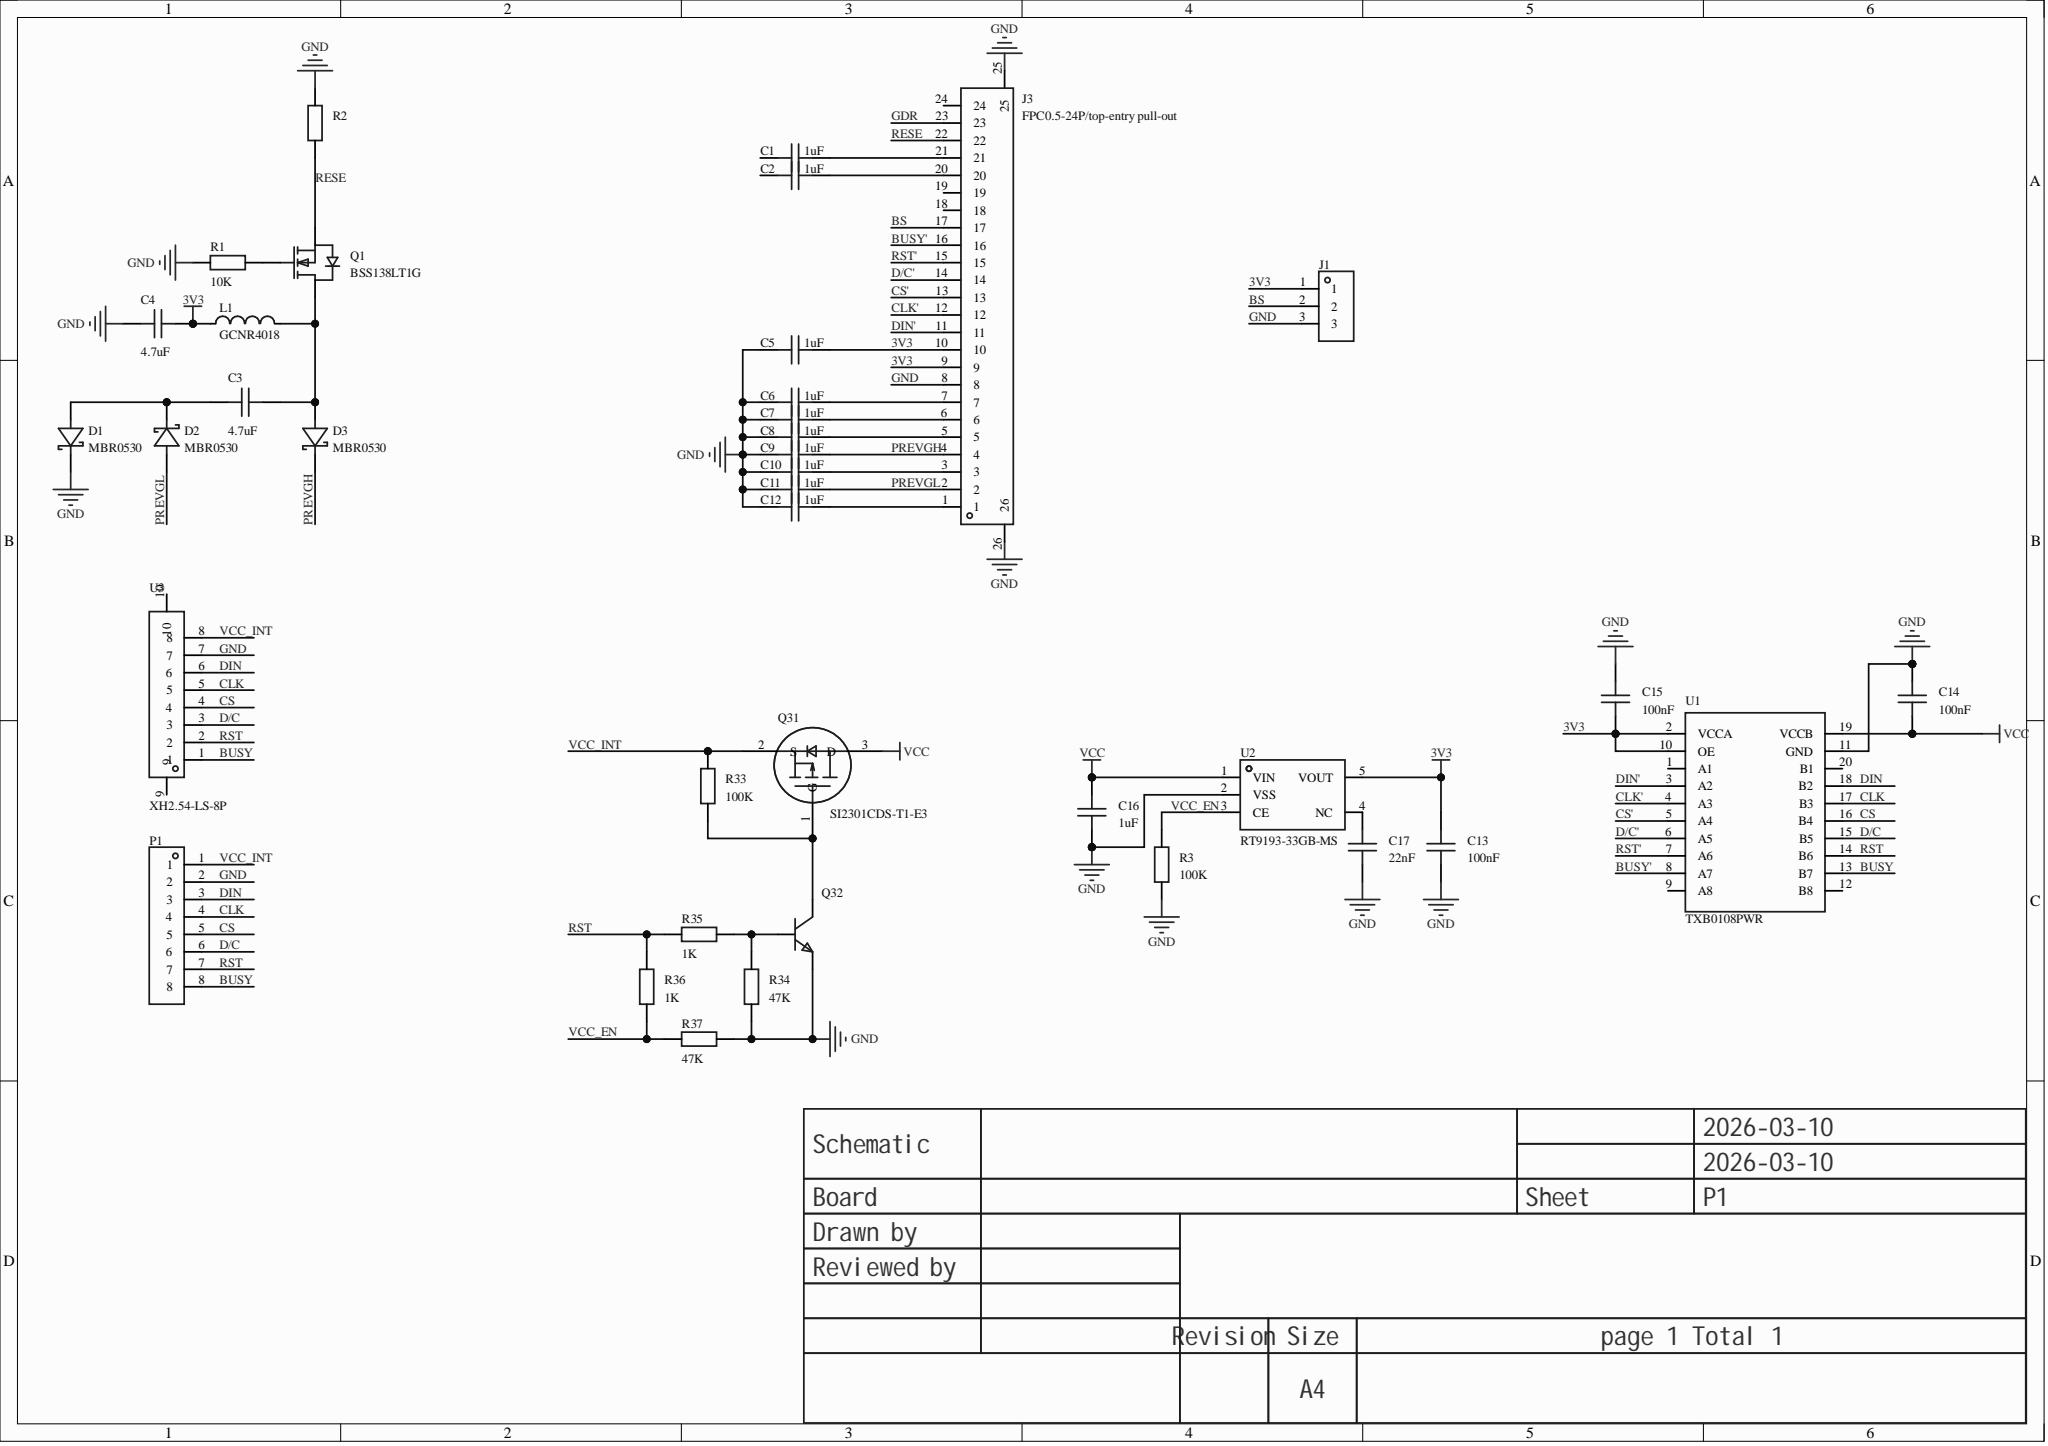Circuit board | Altium Designer | 38 parts | 34 nets
Bill of materials:
Comment,Description,Designator,Footprint,LibRef,Quantity
"1uF","","C1, C2, C5, C6, C7, C8, C9, C10, C11, C12, C16","C0603","CAP_0603","11"
"4.7uF","","C3, C4","C0603","CAP_0603","2"
"100nF","","C13, C14, C15","C0603","CAP_0603","3"
"22nF","","C17","C0603","CAP_0603","1"
"MBR0530","Diode configuration: single; forward voltage (Vf): 550mV@500mA; DC reverse voltage (Vr): 30V; rectified current: 500mA;","D1, D2, D3","SOD-123FL_L2.7-W1.8-LS3.7-RD","MBR0530","3"
"","","J1","HDR-TH_3P-P2.54-V-F","HDR-F_2.54_1x3P","1"
"FPC0.5-24P/top-entry pull-out","","J3","FPC-SMD_24P-P0.50_SHOU-HAN_CTSJ-H2.0","FPC0.5-24P/上接抽拉","1"
"GCNR4018","","L1","IND-SMD_L4.0-W4.0","GCNR4018","1"
"","","P1","HDR-TH_8P-P2.54-V-F-1","HDR-F_2.54_1x8P","1"
"BSS138LT1G","Quantity: 1 N-channel; drain-source voltage (Vdss): 50V; continuous drain current (Id): 200mA; on-resistance (RDS(on)): 5.6O@2.75V; power dissipation (Pd): 225mW; threshold voltage (Vgs(th)): 500mV;","Q1","SOT-23-3_L2.9-W1.6-P1.90-LS2.8-BR","BSS138LT1G","1"
"SI2301CDS-T1-E3","Quantity: 1 P-channel; drain-source voltage (Vdss): 20V; continuous drain current (Id): 3.1A; on-resistance (RDS(on)): 142mO@2.5V,2A; power dissipation (Pd): 1.6W; threshold voltage (Vgs(th)): 1V@250uA;","Q31","SOT-23_L2.9-W1.3-P1.90-LS2.4-BR","SI2301CDS-T1-E3","1"
"","","Q32","S8050_SOT-23","S8050_SOT_NPN","1"
"10K","","R1, R2","R0603","Res_0603","2"
"100K","","R3, R33","R0603","Res_0603","2"
"47K","","R34, R37","R0603","Res_0603","2"
"1K","","R35, R36","R0603","Res_0603","2"
"TXB0108PWR","Data rate: 100Mbps; voltage (VCCA): 1.2V~3.6V; voltage (VCCB): 1.65V~5.5V; number of circuits: 1; channels per circuit: 8;","U1","TSSOP-20_L6.5-W4.4-P0.65-LS6.4-BL","TXB0108PWR","1"
"RT9193-33GB-MS","Output type: fixed; max input voltage: 6V; output voltage: 3.3V; max output current: 300mA; power supply ripple rejection (PSRR): 70dB@(1kHz); output polarity: positive;","U2","SOT-23-5_L2.9-W1.6-P0.95-LS2.8-BR","RT9193-33GB-MS","1"
"XH2.54-LS-8P","","U3","CONN-SMD_XH2.54-LS-8P","XH2.54-LS-8P","1"
Netlist (Protel format):
[
C1
C0603
1uF



]
[
C2
C0603
1uF



]
[
C3
C0603
4.7uF



]
[
C4
C0603
4.7uF



]
[
C5
C0603
1uF



]
[
C6
C0603
1uF



]
[
C7
C0603
1uF



]
[
C8
C0603
1uF



]
[
C9
C0603
1uF



]
[
C10
C0603
1uF



]
[
C11
C0603
1uF



]
[
C12
C0603
1uF



]
[
C13
C0603
100nF



]
[
C14
C0603
100nF



]
[
C15
C0603
100nF



]
[
C16
C0603
1uF



]
[
C17
C0603
22nF



]
[
D1
SOD-123FL_L2.7-W1.8-LS3.7-RD
MBR0530



]
[
D2
SOD-123FL_L2.7-W1.8-LS3.7-RD
MBR0530



]
[
D3
SOD-123FL_L2.7-W1.8-LS3.7-RD
MBR0530



]
[
J1
HDR-TH_3P-P2.54-V-F




]
[
J3
FPC-SMD_24P-P0.50_SHOU-HAN_CTSJ-H2.0
FPC0.5-24P/top-entry pull-out



]
[
L1
IND-SMD_L4.0-W4.0
GCNR4018



]
[
P1
HDR-TH_8P-P2.54-V-F-1




]
[
Q1
SOT-23-3_L2.9-W1.6-P1.90-LS2.8-BR
BSS138LT1G



]
[
Q31
SOT-23_L2.9-W1.3-P1.90-LS2.4-BR
SI2301CDS-T1-E3



]
[
Q32
S8050_SOT-23




]
[
R1
R0603
10K



]
[
R2
R0603
10K



]
[
R3
R0603
100K



]
[
R33
R0603
100K



]
[
R34
R0603
47K



]
[
R35
R0603
1K



]
[
R36
R0603
1K



]
[
R37
R0603
47K



]
[
U1
TSSOP-20_L6.5-W4.4-P0.65-LS6.4-BL
TXB0108PWR



]
[
U2
SOT-23-5_L2.9-W1.6-P0.95-LS2.8-BR
RT9193-33GB-MS



]
[
U3
CONN-SMD_XH2.54-LS-8P
XH2.54-LS-8P



]
(
VCC_INT
P1-1
Q31-2
R33-2
U3-8
)
(
VCC_EN
R3-2
R36-1
R37-1
U2-3
)
(
VCC
C14-1
C16-2
Q31-3
U1-19
U2-1
)
(
RST'
J3-15
U1-7
)
(
RST
P1-7
R35-1
R36-2
U1-14
U3-2
)
(
RESE
J3-22
Q1-2
R2-1
)
(
PREVGL
C11-2
D2-2
J3-2
)
(
PREVGH
C9-2
D3-1
J3-4
)
(
NetQ32_1
Q32-1
R34-2
R35-2
)
(
NetQ31_1
Q31-1
Q32-3
R33-1
)
(
NetQ1_1
Q1-1
R1-1
)
(
NetC17_2
C17-2
U2-4
)
(
NetC12_2
C12-2
J3-1
)
(
NetC10_2
C10-2
J3-3
)
(
NetC8_2
C8-2
J3-5
)
(
NetC7_2
C7-2
J3-6
)
(
NetC6_2
C6-2
J3-7
)
(
NetC3_2
C3-2
D3-2
L1-2
Q1-3
)
(
NetC3_1
C3-1
D1-2
D2-1
)
(
NetC2_2
C2-2
J3-20
)
(
NetC1_2
C1-2
J3-21
)
(
GND
C4-1
C5-1
C6-1
C7-1
C8-1
C9-1
C10-1
C11-1
C12-1
C13-1
C14-2
C15-2
C16-1
C17-1
D1-1
J1-3
J3-8
J3-25
J3-26
P1-2
Q32-2
R1-2
R2-2
R3-1
R34-1
R37-2
U1-11
U2-2
U3-7
)
(
DIN'
J3-11
U1-3
)
(
DIN
P1-3
U1-18
U3-6
)
(
D/C'
J3-14
U1-6
)
(
D/C
P1-6
U1-15
U3-3
)
(
CS'
J3-13
U1-5
)
(
CS
P1-5
U1-16
U3-4
)
(
CLK'
J3-12
U1-4
)
(
CLK
P1-4
U1-17
U3-5
)
(
BUSY'
J3-16
U1-8
)
(
BUSY
P1-8
U1-13
U3-1
)
(
BS
J1-2
J3-17
)
(
3V3
C4-2
C5-2
C13-2
C15-1
J1-1
J3-9
J3-10
L1-1
U1-2
U1-10
U2-5
)